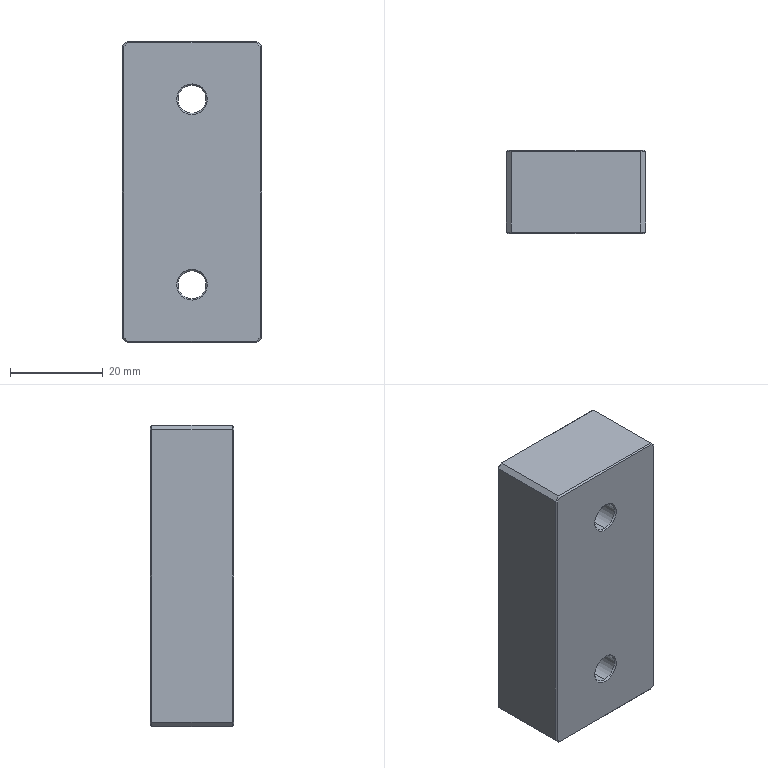Part | STEP file | lifting air cylinder fixing support seat 03 | 1 solid | 38 faces | box 30 x 18 x 65 mm | volume 34026 mm3 | plane 26 | cone 8 | cylinder 4 | commonest cylinder face diameters 6 x4